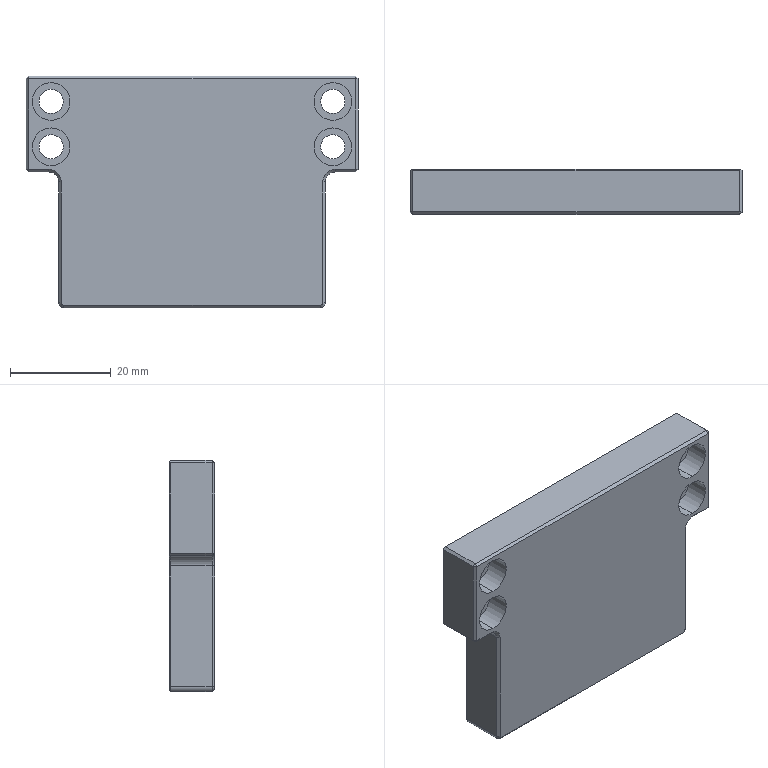Part | SolidWorks | features BaseBody 1 | 1 solid | 66 faces | box 66 x 9 x 46 mm | volume 23009 mm3 | plane 38 | cylinder 20 | cone 8 | commonest cylinder face diameters 4.8 x8 7.5 x8 2 x2 4 x2